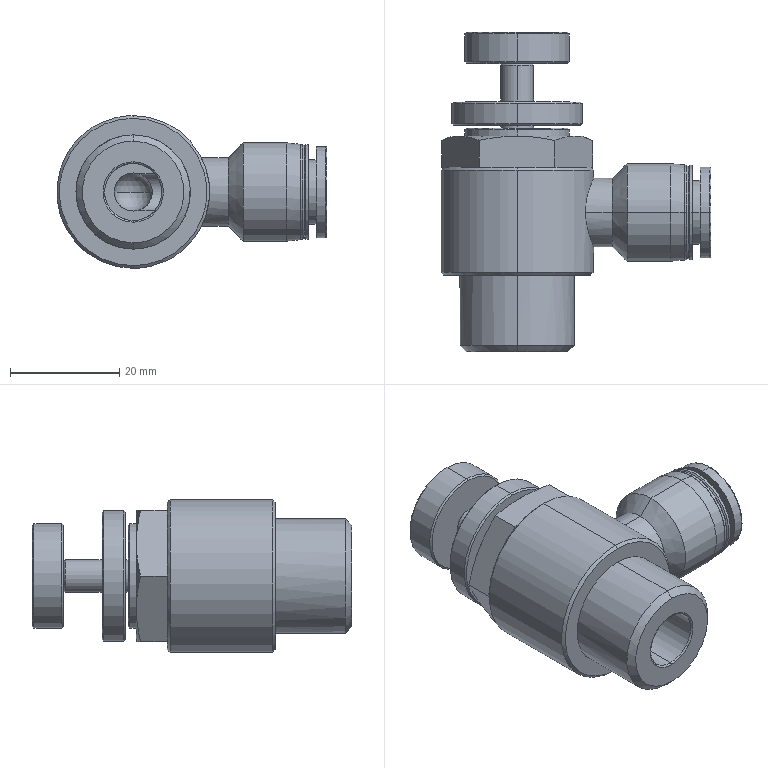Part | SolidWorks | features BaseBody 1 | 1 solid | 120 faces | box 49.5 x 58.5 x 28 mm | volume 24100 mm3 | plane 44 | cylinder 36 | cone 32 | torus 6 | sphere 2 | commonest cylinder face diameters 6 x4 17.4 x4 19.2 x4 6.667 x2 6.985 x2 10 x2